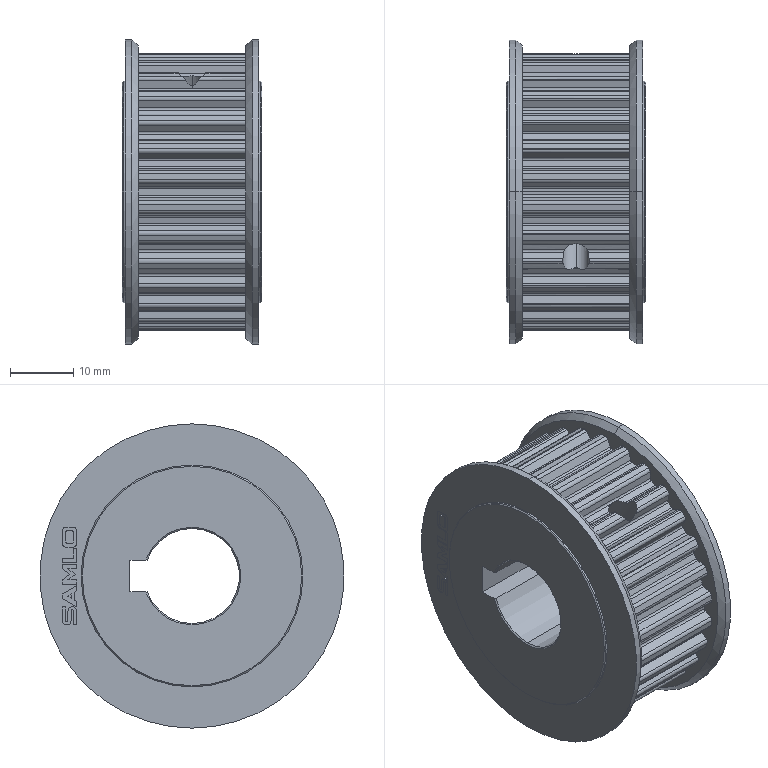Part | STEP file | 1 solid | 365 faces | box 22 x 48 x 48 mm | volume 27125 mm3 | cylinder 233 | plane 120 | cone 12 | commonest cylinder face diameters 1.2 x73 0.8 x71 40.15 x31 43.75 x29 0.523 x4 1.108 x4